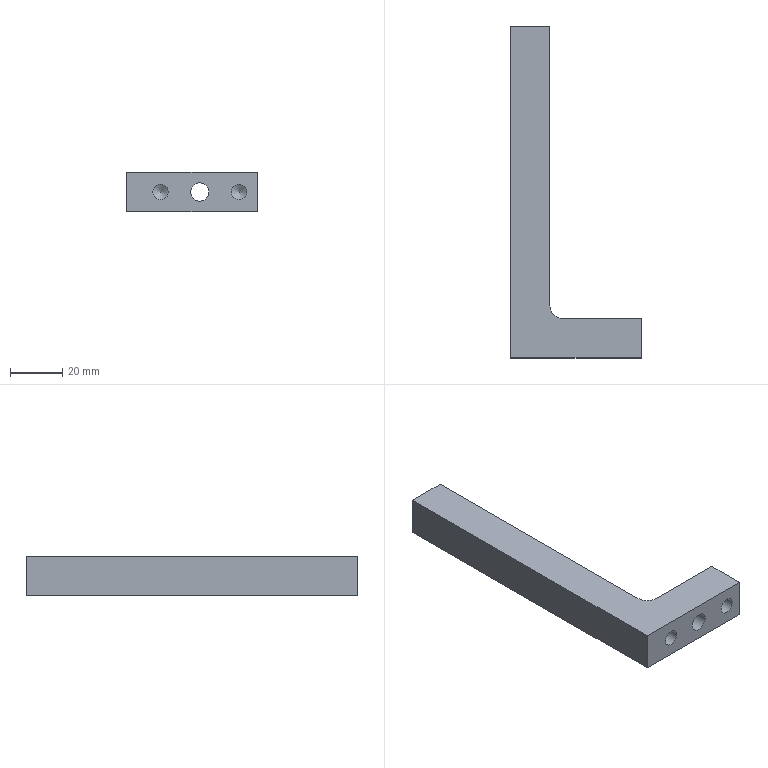Part | NX | features BREP 1 | 1 solid | 16 faces | box 50 x 127 x 15 mm | volume 34499 mm3 | plane 8 | cylinder 5 | cone 3 | commonest cylinder face diameters 6 x2 6.8 x1 7 x1 10 x1
STEP:
#1=CARTESIAN_POINT('',(16.5,0.,7.5));
#2=VERTEX_POINT('',#1);
#3=CARTESIAN_POINT('',(13.,0.,7.5));
#4=DIRECTION('',(0.,-1.,0.));
#5=DIRECTION('',(1.,0.,0.));
#6=AXIS2_PLACEMENT_3D('',#3,#4,#5);
#7=CIRCLE('',#6,3.5);
#8=EDGE_CURVE('',#2,#2,#7,.T.);
#9=ORIENTED_EDGE('',*,*,#8,.T.);
#10=EDGE_LOOP('',(#9));
#11=FACE_BOUND('',#10,.T.);
#12=CARTESIAN_POINT('',(35.,0.,0.));
#13=VERTEX_POINT('',#12);
#14=CARTESIAN_POINT('',(5.,0.,0.));
#15=VERTEX_POINT('',#14);
#16=CARTESIAN_POINT('',(35.,0.,0.));
#17=DIRECTION('',(-1.,0.,0.));
#18=VECTOR('',#17,1000.);
#19=LINE('',#16,#18);
#20=EDGE_CURVE('',#13,#15,#19,.T.);
#21=ORIENTED_EDGE('',*,*,#20,.T.);
#22=CARTESIAN_POINT('',(5.,0.,15.));
#23=VERTEX_POINT('',#22);
#24=CARTESIAN_POINT('',(5.,0.,15.));
#25=DIRECTION('',(0.,0.,1.));
#26=VECTOR('',#25,1000.);
#27=LINE('',#24,#26);
#28=EDGE_CURVE('',#15,#23,#27,.T.);
#29=ORIENTED_EDGE('',*,*,#28,.T.);
#30=CARTESIAN_POINT('',(35.,0.,15.));
#31=VERTEX_POINT('',#30);
#32=CARTESIAN_POINT('',(35.,0.,15.));
#33=DIRECTION('',(-1.,0.,0.));
#34=VECTOR('',#33,1000.);
#35=LINE('',#32,#34);
#36=EDGE_CURVE('',#31,#23,#35,.T.);
#37=ORIENTED_EDGE('',*,*,#36,.F.);
#38=CARTESIAN_POINT('',(35.,0.,15.));
#39=DIRECTION('',(0.,0.,-1.));
#40=VECTOR('',#39,1000.);
#41=LINE('',#38,#40);
#42=EDGE_CURVE('',#31,#13,#41,.T.);
#43=ORIENTED_EDGE('',*,*,#42,.T.);
#44=EDGE_LOOP('',(#21,#29,#37,#43));
#45=FACE_BOUND('',#44,.T.);
#46=CARTESIAN_POINT('',(35.,0.,15.));
#47=DIRECTION('',(0.,-1.,0.));
#48=DIRECTION('',(-1.,0.,0.));
#49=AXIS2_PLACEMENT_3D('',#46,#47,#48);
#50=PLANE('',#49);
#51=ADVANCED_FACE('',(#11,#45),#50,.F.);
#52=CARTESIAN_POINT('',(0.,5.,15.));
#53=VERTEX_POINT('',#52);
#54=CARTESIAN_POINT('',(0.,112.,15.));
#55=VERTEX_POINT('',#54);
#56=CARTESIAN_POINT('',(0.,0.,15.));
#57=DIRECTION('',(0.,1.,0.));
#58=VECTOR('',#57,1000.);
#59=LINE('',#56,#58);
#60=EDGE_CURVE('',#53,#55,#59,.T.);
#61=ORIENTED_EDGE('',*,*,#60,.F.);
#62=CARTESIAN_POINT('',(0.,5.,0.));
#63=VERTEX_POINT('',#62);
#64=CARTESIAN_POINT('',(0.,5.,0.));
#65=DIRECTION('',(0.,0.,-1.));
#66=VECTOR('',#65,1000.);
#67=LINE('',#64,#66);
#68=EDGE_CURVE('',#53,#63,#67,.T.);
#69=ORIENTED_EDGE('',*,*,#68,.T.);
#70=CARTESIAN_POINT('',(0.,112.,0.));
#71=VERTEX_POINT('',#70);
#72=CARTESIAN_POINT('',(0.,0.,0.));
#73=DIRECTION('',(0.,1.,0.));
#74=VECTOR('',#73,1000.);
#75=LINE('',#72,#74);
#76=EDGE_CURVE('',#63,#71,#75,.T.);
#77=ORIENTED_EDGE('',*,*,#76,.T.);
#78=CARTESIAN_POINT('',(0.,112.,15.));
#79=DIRECTION('',(0.,0.,-1.));
#80=VECTOR('',#79,1000.);
#81=LINE('',#78,#80);
#82=EDGE_CURVE('',#55,#71,#81,.T.);
#83=ORIENTED_EDGE('',*,*,#82,.F.);
#84=EDGE_LOOP('',(#61,#69,#77,#83));
#85=FACE_BOUND('',#84,.T.);
#86=CARTESIAN_POINT('',(0.,0.,15.));
#87=DIRECTION('',(-1.,0.,0.));
#88=DIRECTION('',(0.,1.,0.));
#89=AXIS2_PLACEMENT_3D('',#86,#87,#88);
#90=PLANE('',#89);
#91=ADVANCED_FACE('',(#85),#90,.F.);
#92=CARTESIAN_POINT('',(-7.5,112.,10.9));
#93=VERTEX_POINT('',#92);
#94=CARTESIAN_POINT('',(-7.5,112.,7.5));
#95=DIRECTION('',(0.,1.,0.));
#96=DIRECTION('',(0.,0.,1.));
#97=AXIS2_PLACEMENT_3D('',#94,#95,#96);
#98=CIRCLE('',#97,3.4);
#99=EDGE_CURVE('',#93,#93,#98,.T.);
#100=ORIENTED_EDGE('',*,*,#99,.F.);
#101=EDGE_LOOP('',(#100));
#102=FACE_BOUND('',#101,.T.);
#103=CARTESIAN_POINT('',(-15.,112.,0.));
#104=VERTEX_POINT('',#103);
#105=CARTESIAN_POINT('',(0.,112.,0.));
#106=DIRECTION('',(-1.,0.,0.));
#107=VECTOR('',#106,1000.);
#108=LINE('',#105,#107);
#109=EDGE_CURVE('',#71,#104,#108,.T.);
#110=ORIENTED_EDGE('',*,*,#109,.T.);
#111=CARTESIAN_POINT('',(-15.,112.,15.));
#112=VERTEX_POINT('',#111);
#113=CARTESIAN_POINT('',(-15.,112.,15.));
#114=DIRECTION('',(0.,0.,-1.));
#115=VECTOR('',#114,1000.);
#116=LINE('',#113,#115);
#117=EDGE_CURVE('',#112,#104,#116,.T.);
#118=ORIENTED_EDGE('',*,*,#117,.F.);
#119=CARTESIAN_POINT('',(0.,112.,15.));
#120=DIRECTION('',(-1.,0.,0.));
#121=VECTOR('',#120,1000.);
#122=LINE('',#119,#121);
#123=EDGE_CURVE('',#55,#112,#122,.T.);
#124=ORIENTED_EDGE('',*,*,#123,.F.);
#125=ORIENTED_EDGE('',*,*,#82,.T.);
#126=EDGE_LOOP('',(#110,#118,#124,#125));
#127=FACE_BOUND('',#126,.T.);
#128=CARTESIAN_POINT('',(0.,112.,15.));
#129=DIRECTION('',(0.,-1.,0.));
#130=DIRECTION('',(0.,0.,1.));
#131=AXIS2_PLACEMENT_3D('',#128,#129,#130);
#132=PLANE('',#131);
#133=ADVANCED_FACE('',(#102,#127),#132,.F.);
#134=CARTESIAN_POINT('',(-15.,-15.,0.));
#135=VERTEX_POINT('',#134);
#136=CARTESIAN_POINT('',(-15.,112.,0.));
#137=DIRECTION('',(0.,-1.,0.));
#138=VECTOR('',#137,1000.);
#139=LINE('',#136,#138);
#140=EDGE_CURVE('',#104,#135,#139,.T.);
#141=ORIENTED_EDGE('',*,*,#140,.T.);
#142=CARTESIAN_POINT('',(-15.,-15.,15.));
#143=VERTEX_POINT('',#142);
#144=CARTESIAN_POINT('',(-15.,-15.,15.));
#145=DIRECTION('',(0.,0.,-1.));
#146=VECTOR('',#145,1000.);
#147=LINE('',#144,#146);
#148=EDGE_CURVE('',#143,#135,#147,.T.);
#149=ORIENTED_EDGE('',*,*,#148,.F.);
#150=CARTESIAN_POINT('',(-15.,112.,15.));
#151=DIRECTION('',(0.,-1.,0.));
#152=VECTOR('',#151,1000.);
#153=LINE('',#150,#152);
#154=EDGE_CURVE('',#112,#143,#153,.T.);
#155=ORIENTED_EDGE('',*,*,#154,.F.);
#156=ORIENTED_EDGE('',*,*,#117,.T.);
#157=EDGE_LOOP('',(#141,#149,#155,#156));
#158=FACE_BOUND('',#157,.T.);
#159=CARTESIAN_POINT('',(-15.,112.,15.));
#160=DIRECTION('',(1.,0.,0.));
#161=DIRECTION('',(0.,-1.,0.));
#162=AXIS2_PLACEMENT_3D('',#159,#160,#161);
#163=PLANE('',#162);
#164=ADVANCED_FACE('',(#158),#163,.F.);
#165=CARTESIAN_POINT('',(13.,-15.,4.));
#166=VERTEX_POINT('',#165);
#167=CARTESIAN_POINT('',(13.,-15.,7.5));
#168=DIRECTION('',(0.,-1.,0.));
#169=DIRECTION('',(0.,0.,-1.));
#170=AXIS2_PLACEMENT_3D('',#167,#168,#169);
#171=CIRCLE('',#170,3.5);
#172=EDGE_CURVE('',#166,#166,#171,.T.);
#173=ORIENTED_EDGE('',*,*,#172,.F.);
#174=EDGE_LOOP('',(#173));
#175=FACE_BOUND('',#174,.T.);
#176=CARTESIAN_POINT('',(28.,-15.,4.5));
#177=VERTEX_POINT('',#176);
#178=CARTESIAN_POINT('',(28.,-15.,7.5));
#179=DIRECTION('',(0.,-1.,0.));
#180=DIRECTION('',(0.,0.,-1.));
#181=AXIS2_PLACEMENT_3D('',#178,#179,#180);
#182=CIRCLE('',#181,3.);
#183=EDGE_CURVE('',#177,#177,#182,.T.);
#184=ORIENTED_EDGE('',*,*,#183,.F.);
#185=EDGE_LOOP('',(#184));
#186=FACE_BOUND('',#185,.T.);
#187=CARTESIAN_POINT('',(-2.,-15.,4.5));
#188=VERTEX_POINT('',#187);
#189=CARTESIAN_POINT('',(-2.,-15.,7.5));
#190=DIRECTION('',(0.,-1.,0.));
#191=DIRECTION('',(0.,0.,-1.));
#192=AXIS2_PLACEMENT_3D('',#189,#190,#191);
#193=CIRCLE('',#192,3.);
#194=EDGE_CURVE('',#188,#188,#193,.T.);
#195=ORIENTED_EDGE('',*,*,#194,.F.);
#196=EDGE_LOOP('',(#195));
#197=FACE_BOUND('',#196,.T.);
#198=CARTESIAN_POINT('',(35.,-15.,0.));
#199=VERTEX_POINT('',#198);
#200=CARTESIAN_POINT('',(-15.,-15.,0.));
#201=DIRECTION('',(1.,0.,0.));
#202=VECTOR('',#201,1000.);
#203=LINE('',#200,#202);
#204=EDGE_CURVE('',#135,#199,#203,.T.);
#205=ORIENTED_EDGE('',*,*,#204,.T.);
#206=CARTESIAN_POINT('',(35.,-15.,15.));
#207=VERTEX_POINT('',#206);
#208=CARTESIAN_POINT('',(35.,-15.,15.));
#209=DIRECTION('',(0.,0.,-1.));
#210=VECTOR('',#209,1000.);
#211=LINE('',#208,#210);
#212=EDGE_CURVE('',#207,#199,#211,.T.);
#213=ORIENTED_EDGE('',*,*,#212,.F.);
#214=CARTESIAN_POINT('',(-15.,-15.,15.));
#215=DIRECTION('',(1.,0.,0.));
#216=VECTOR('',#215,1000.);
#217=LINE('',#214,#216);
#218=EDGE_CURVE('',#143,#207,#217,.T.);
#219=ORIENTED_EDGE('',*,*,#218,.F.);
#220=ORIENTED_EDGE('',*,*,#148,.T.);
#221=EDGE_LOOP('',(#205,#213,#219,#220));
#222=FACE_BOUND('',#221,.T.);
#223=CARTESIAN_POINT('',(-15.,-15.,15.));
#224=DIRECTION('',(0.,1.,0.));
#225=DIRECTION('',(1.,0.,0.));
#226=AXIS2_PLACEMENT_3D('',#223,#224,#225);
#227=PLANE('',#226);
#228=ADVANCED_FACE('',(#175,#186,#197,#222),#227,.F.);
#229=CARTESIAN_POINT('',(35.,-15.,0.));
#230=DIRECTION('',(0.,1.,0.));
#231=VECTOR('',#230,1000.);
#232=LINE('',#229,#231);
#233=EDGE_CURVE('',#199,#13,#232,.T.);
#234=ORIENTED_EDGE('',*,*,#233,.T.);
#235=ORIENTED_EDGE('',*,*,#42,.F.);
#236=CARTESIAN_POINT('',(35.,-15.,15.));
#237=DIRECTION('',(0.,1.,0.));
#238=VECTOR('',#237,1000.);
#239=LINE('',#236,#238);
#240=EDGE_CURVE('',#207,#31,#239,.T.);
#241=ORIENTED_EDGE('',*,*,#240,.F.);
#242=ORIENTED_EDGE('',*,*,#212,.T.);
#243=EDGE_LOOP('',(#234,#235,#241,#242));
#244=FACE_BOUND('',#243,.T.);
#245=CARTESIAN_POINT('',(35.,-15.,15.));
#246=DIRECTION('',(-1.,0.,0.));
#247=DIRECTION('',(0.,0.,-1.));
#248=AXIS2_PLACEMENT_3D('',#245,#246,#247);
#249=PLANE('',#248);
#250=ADVANCED_FACE('',(#244),#249,.F.);
#251=ORIENTED_EDGE('',*,*,#36,.T.);
#252=CARTESIAN_POINT('',(5.,5.,15.));
#253=DIRECTION('',(0.,0.,-1.));
#254=DIRECTION('',(-1.,0.,0.));
#255=AXIS2_PLACEMENT_3D('',#252,#253,#254);
#256=CIRCLE('',#255,5.);
#257=EDGE_CURVE('',#23,#53,#256,.T.);
#258=ORIENTED_EDGE('',*,*,#257,.T.);
#259=ORIENTED_EDGE('',*,*,#60,.T.);
#260=ORIENTED_EDGE('',*,*,#123,.T.);
#261=ORIENTED_EDGE('',*,*,#154,.T.);
#262=ORIENTED_EDGE('',*,*,#218,.T.);
#263=ORIENTED_EDGE('',*,*,#240,.T.);
#264=EDGE_LOOP('',(#251,#258,#259,#260,#261,#262,#263));
#265=FACE_BOUND('',#264,.T.);
#266=CARTESIAN_POINT('',(0.,0.,15.));
#267=DIRECTION('',(0.,0.,-1.));
#268=DIRECTION('',(1.,0.,0.));
#269=AXIS2_PLACEMENT_3D('',#266,#267,#268);
#270=PLANE('',#269);
#271=ADVANCED_FACE('',(#265),#270,.F.);
#272=ORIENTED_EDGE('',*,*,#20,.F.);
#273=ORIENTED_EDGE('',*,*,#233,.F.);
#274=ORIENTED_EDGE('',*,*,#204,.F.);
#275=ORIENTED_EDGE('',*,*,#140,.F.);
#276=ORIENTED_EDGE('',*,*,#109,.F.);
#277=ORIENTED_EDGE('',*,*,#76,.F.);
#278=CARTESIAN_POINT('',(5.,5.,0.));
#279=DIRECTION('',(0.,0.,1.));
#280=DIRECTION('',(-1.,0.,0.));
#281=AXIS2_PLACEMENT_3D('',#278,#279,#280);
#282=CIRCLE('',#281,5.);
#283=EDGE_CURVE('',#63,#15,#282,.T.);
#284=ORIENTED_EDGE('',*,*,#283,.T.);
#285=EDGE_LOOP('',(#272,#273,#274,#275,#276,#277,#284));
#286=FACE_BOUND('',#285,.T.);
#287=CARTESIAN_POINT('',(0.,0.,0.));
#288=DIRECTION('',(0.,0.,-1.));
#289=DIRECTION('',(1.,0.,0.));
#290=AXIS2_PLACEMENT_3D('',#287,#288,#289);
#291=PLANE('',#290);
#292=ADVANCED_FACE('',(#286),#291,.T.);
#293=ORIENTED_EDGE('',*,*,#257,.F.);
#294=ORIENTED_EDGE('',*,*,#28,.F.);
#295=ORIENTED_EDGE('',*,*,#283,.F.);
#296=ORIENTED_EDGE('',*,*,#68,.F.);
#297=EDGE_LOOP('',(#293,#294,#295,#296));
#298=FACE_BOUND('',#297,.T.);
#299=CARTESIAN_POINT('',(5.,5.,15.));
#300=DIRECTION('',(0.,0.,1.));
#301=DIRECTION('',(-1.,0.,0.));
#302=AXIS2_PLACEMENT_3D('',#299,#300,#301);
#303=CYLINDRICAL_SURFACE('',#302,5.);
#304=ADVANCED_FACE('',(#298),#303,.F.);
#305=CARTESIAN_POINT('',(-2.,-1.197,7.5));
#306=VERTEX_POINT('',#305);
#307=VERTEX_LOOP('',#306);
#308=FACE_BOUND('',#307,.T.);
#309=CARTESIAN_POINT('',(-2.,-3.,4.5));
#310=VERTEX_POINT('',#309);
#311=CARTESIAN_POINT('',(-2.,-3.,7.5));
#312=DIRECTION('',(0.,-1.,0.));
#313=DIRECTION('',(0.,0.,-1.));
#314=AXIS2_PLACEMENT_3D('',#311,#312,#313);
#315=CIRCLE('',#314,3.);
#316=EDGE_CURVE('',#310,#310,#315,.T.);
#317=ORIENTED_EDGE('',*,*,#316,.T.);
#318=EDGE_LOOP('',(#317));
#319=FACE_BOUND('',#318,.T.);
#320=CARTESIAN_POINT('',(-2.,-3.,7.5));
#321=DIRECTION('',(0.,-1.,0.));
#322=DIRECTION('',(0.,0.,1.));
#323=AXIS2_PLACEMENT_3D('',#320,#321,#322);
#324=CONICAL_SURFACE('',#323,3.,1.03);
#325=ADVANCED_FACE('',(#308,#319),#324,.F.);
#326=ORIENTED_EDGE('',*,*,#316,.F.);
#327=EDGE_LOOP('',(#326));
#328=FACE_BOUND('',#327,.T.);
#329=ORIENTED_EDGE('',*,*,#194,.T.);
#330=EDGE_LOOP('',(#329));
#331=FACE_BOUND('',#330,.T.);
#332=CARTESIAN_POINT('',(-2.,-15.,7.5));
#333=DIRECTION('',(0.,-1.,0.));
#334=DIRECTION('',(0.,0.,1.));
#335=AXIS2_PLACEMENT_3D('',#332,#333,#334);
#336=CYLINDRICAL_SURFACE('',#335,3.);
#337=ADVANCED_FACE('',(#328,#331),#336,.F.);
#338=CARTESIAN_POINT('',(28.,-1.197,7.5));
#339=VERTEX_POINT('',#338);
#340=VERTEX_LOOP('',#339);
#341=FACE_BOUND('',#340,.T.);
#342=CARTESIAN_POINT('',(28.,-3.,4.5));
#343=VERTEX_POINT('',#342);
#344=CARTESIAN_POINT('',(28.,-3.,7.5));
#345=DIRECTION('',(0.,-1.,0.));
#346=DIRECTION('',(0.,0.,-1.));
#347=AXIS2_PLACEMENT_3D('',#344,#345,#346);
#348=CIRCLE('',#347,3.);
#349=EDGE_CURVE('',#343,#343,#348,.T.);
#350=ORIENTED_EDGE('',*,*,#349,.T.);
#351=EDGE_LOOP('',(#350));
#352=FACE_BOUND('',#351,.T.);
#353=CARTESIAN_POINT('',(28.,-3.,7.5));
#354=DIRECTION('',(0.,-1.,0.));
#355=DIRECTION('',(0.,0.,1.));
#356=AXIS2_PLACEMENT_3D('',#353,#354,#355);
#357=CONICAL_SURFACE('',#356,3.,1.03);
#358=ADVANCED_FACE('',(#341,#352),#357,.F.);
#359=ORIENTED_EDGE('',*,*,#349,.F.);
#360=EDGE_LOOP('',(#359));
#361=FACE_BOUND('',#360,.T.);
#362=ORIENTED_EDGE('',*,*,#183,.T.);
#363=EDGE_LOOP('',(#362));
#364=FACE_BOUND('',#363,.T.);
#365=CARTESIAN_POINT('',(28.,-15.,7.5));
#366=DIRECTION('',(0.,-1.,0.));
#367=DIRECTION('',(0.,0.,1.));
#368=AXIS2_PLACEMENT_3D('',#365,#366,#367);
#369=CYLINDRICAL_SURFACE('',#368,3.);
#370=ADVANCED_FACE('',(#361,#364),#369,.F.);
#371=ORIENTED_EDGE('',*,*,#172,.T.);
#372=EDGE_LOOP('',(#371));
#373=FACE_BOUND('',#372,.T.);
#374=ORIENTED_EDGE('',*,*,#8,.F.);
#375=EDGE_LOOP('',(#374));
#376=FACE_BOUND('',#375,.T.);
#377=CARTESIAN_POINT('',(13.,-15.,7.5));
#378=DIRECTION('',(0.,-1.,0.));
#379=DIRECTION('',(0.,0.,1.));
#380=AXIS2_PLACEMENT_3D('',#377,#378,#379);
#381=CYLINDRICAL_SURFACE('',#380,3.5);
#382=ADVANCED_FACE('',(#373,#376),#381,.F.);
#383=CARTESIAN_POINT('',(-7.5,90.207,7.5));
#384=VERTEX_POINT('',#383);
#385=VERTEX_LOOP('',#384);
#386=FACE_BOUND('',#385,.T.);
#387=CARTESIAN_POINT('',(-7.5,92.25,10.9));
#388=VERTEX_POINT('',#387);
#389=CARTESIAN_POINT('',(-7.5,92.25,7.5));
#390=DIRECTION('',(0.,1.,0.));
#391=DIRECTION('',(0.,0.,1.));
#392=AXIS2_PLACEMENT_3D('',#389,#390,#391);
#393=CIRCLE('',#392,3.4);
#394=EDGE_CURVE('',#388,#388,#393,.T.);
#395=ORIENTED_EDGE('',*,*,#394,.T.);
#396=EDGE_LOOP('',(#395));
#397=FACE_BOUND('',#396,.T.);
#398=CARTESIAN_POINT('',(-7.5,92.25,7.5));
#399=DIRECTION('',(0.,1.,0.));
#400=DIRECTION('',(0.,0.,-1.));
#401=AXIS2_PLACEMENT_3D('',#398,#399,#400);
#402=CONICAL_SURFACE('',#401,3.4,1.03);
#403=ADVANCED_FACE('',(#386,#397),#402,.F.);
#404=ORIENTED_EDGE('',*,*,#394,.F.);
#405=EDGE_LOOP('',(#404));
#406=FACE_BOUND('',#405,.T.);
#407=ORIENTED_EDGE('',*,*,#99,.T.);
#408=EDGE_LOOP('',(#407));
#409=FACE_BOUND('',#408,.T.);
#410=CARTESIAN_POINT('',(-7.5,112.,7.5));
#411=DIRECTION('',(0.,1.,0.));
#412=DIRECTION('',(0.,0.,-1.));
#413=AXIS2_PLACEMENT_3D('',#410,#411,#412);
#414=CYLINDRICAL_SURFACE('',#413,3.4);
#415=ADVANCED_FACE('',(#406,#409),#414,.F.);
#416=CLOSED_SHELL('',(#51,#91,#133,#164,#228,#250,#271,#292,#304,#325,#337,#358,#370,#382,#403,#415));
#417=MANIFOLD_SOLID_BREP('',#416);
#418=(LENGTH_UNIT()NAMED_UNIT(*)SI_UNIT(.MILLI.,.METRE.));
#419=UNCERTAINTY_MEASURE_WITH_UNIT(LENGTH_MEASURE(0.00001),#418,'','');
#420=(NAMED_UNIT(*)PLANE_ANGLE_UNIT()SI_UNIT($,.RADIAN.));
#421=(NAMED_UNIT(*)SI_UNIT($,.STERADIAN.)SOLID_ANGLE_UNIT());
#422=(GEOMETRIC_REPRESENTATION_CONTEXT(3)GLOBAL_UNCERTAINTY_ASSIGNED_CONTEXT((#419))GLOBAL_UNIT_ASSIGNED_CONTEXT((#418,#420,#421))REPRESENTATION_CONTEXT('',''));
#423=ADVANCED_BREP_SHAPE_REPRESENTATION('',(#417),#422);